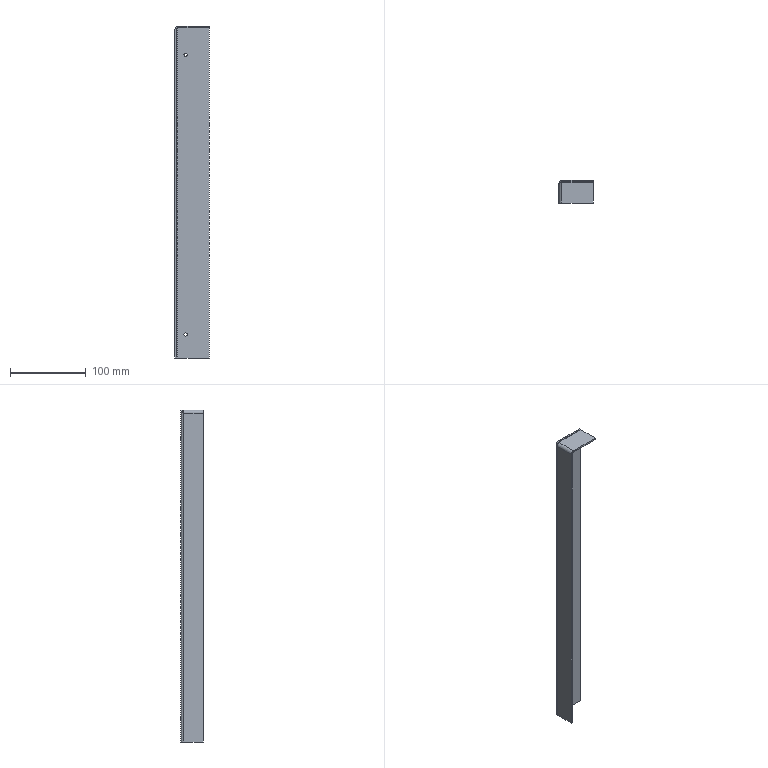Part | STEP file | SYL_0392D6J1SYL0380DJ100-288319 | 1 solid | 26 faces | box 45 x 30 x 438 mm | volume 65045 mm3 | plane 16 | cylinder 8 | spline 2 | commonest cylinder face diameters 4.2 x4 4 x2 8 x2
STEP:
#1=CARTESIAN_POINT('',(-8.5,28.,-190.1));
#2=VERTEX_POINT('',#1);
#3=CARTESIAN_POINT('',(-8.5,30.,-190.1));
#4=VERTEX_POINT('',#3);
#5=CARTESIAN_POINT('',(-8.5,30.,-190.1));
#6=DIRECTION('',(0.,1.,0.));
#7=VECTOR('',#6,1000.);
#8=LINE('',#5,#7);
#9=EDGE_CURVE('',#2,#4,#8,.T.);
#10=ORIENTED_EDGE('',*,*,#9,.F.);
#11=CARTESIAN_POINT('',(-8.5,28.,-185.9));
#12=VERTEX_POINT('',#11);
#13=CARTESIAN_POINT('',(-8.5,28.,-188.));
#14=DIRECTION('',(0.,-1.,0.));
#15=DIRECTION('',(0.,0.,-1.));
#16=AXIS2_PLACEMENT_3D('',#13,#14,#15);
#17=CIRCLE('',#16,2.1);
#18=EDGE_CURVE('',#2,#12,#17,.T.);
#19=ORIENTED_EDGE('',*,*,#18,.T.);
#20=CARTESIAN_POINT('',(-8.5,30.,-185.9));
#21=VERTEX_POINT('',#20);
#22=CARTESIAN_POINT('',(-8.5,30.,-185.9));
#23=DIRECTION('',(0.,1.,0.));
#24=VECTOR('',#23,1000.);
#25=LINE('',#22,#24);
#26=EDGE_CURVE('',#12,#21,#25,.T.);
#27=ORIENTED_EDGE('',*,*,#26,.T.);
#28=CARTESIAN_POINT('',(-8.5,30.,-188.));
#29=DIRECTION('',(0.,-1.,0.));
#30=DIRECTION('',(0.,0.,-1.));
#31=AXIS2_PLACEMENT_3D('',#28,#29,#30);
#32=CIRCLE('',#31,2.1);
#33=EDGE_CURVE('',#4,#21,#32,.T.);
#34=ORIENTED_EDGE('',*,*,#33,.F.);
#35=EDGE_LOOP('',(#10,#19,#27,#34));
#36=FACE_OUTER_BOUND('',#35,.T.);
#37=CARTESIAN_POINT('',(-8.5,30.,-188.));
#38=DIRECTION('',(0.,1.,0.));
#39=DIRECTION('',(0.,0.,1.));
#40=AXIS2_PLACEMENT_3D('',#37,#38,#39);
#41=CYLINDRICAL_SURFACE('',#40,2.1);
#42=ADVANCED_FACE('',(#36),#41,.F.);
#43=CARTESIAN_POINT('',(-8.5,28.,178.9));
#44=VERTEX_POINT('',#43);
#45=CARTESIAN_POINT('',(-8.5,30.,178.9));
#46=VERTEX_POINT('',#45);
#47=CARTESIAN_POINT('',(-8.5,30.,178.9));
#48=DIRECTION('',(0.,1.,0.));
#49=VECTOR('',#48,1000.);
#50=LINE('',#47,#49);
#51=EDGE_CURVE('',#44,#46,#50,.T.);
#52=ORIENTED_EDGE('',*,*,#51,.F.);
#53=CARTESIAN_POINT('',(-8.5,28.,183.1));
#54=VERTEX_POINT('',#53);
#55=CARTESIAN_POINT('',(-8.5,28.,181.));
#56=DIRECTION('',(0.,-1.,0.));
#57=DIRECTION('',(0.,0.,-1.));
#58=AXIS2_PLACEMENT_3D('',#55,#56,#57);
#59=CIRCLE('',#58,2.1);
#60=EDGE_CURVE('',#44,#54,#59,.T.);
#61=ORIENTED_EDGE('',*,*,#60,.T.);
#62=CARTESIAN_POINT('',(-8.5,30.,183.1));
#63=VERTEX_POINT('',#62);
#64=CARTESIAN_POINT('',(-8.5,30.,183.1));
#65=DIRECTION('',(0.,1.,0.));
#66=VECTOR('',#65,1000.);
#67=LINE('',#64,#66);
#68=EDGE_CURVE('',#54,#63,#67,.T.);
#69=ORIENTED_EDGE('',*,*,#68,.T.);
#70=CARTESIAN_POINT('',(-8.5,30.,181.));
#71=DIRECTION('',(0.,-1.,0.));
#72=DIRECTION('',(0.,0.,-1.));
#73=AXIS2_PLACEMENT_3D('',#70,#71,#72);
#74=CIRCLE('',#73,2.1);
#75=EDGE_CURVE('',#46,#63,#74,.T.);
#76=ORIENTED_EDGE('',*,*,#75,.F.);
#77=EDGE_LOOP('',(#52,#61,#69,#76));
#78=FACE_OUTER_BOUND('',#77,.T.);
#79=CARTESIAN_POINT('',(-8.5,30.,181.));
#80=DIRECTION('',(0.,1.,0.));
#81=DIRECTION('',(0.,0.,1.));
#82=AXIS2_PLACEMENT_3D('',#79,#80,#81);
#83=CYLINDRICAL_SURFACE('',#82,2.1);
#84=ADVANCED_FACE('',(#78),#83,.F.);
#85=CARTESIAN_POINT('',(-18.5,28.,219.));
#86=VERTEX_POINT('',#85);
#87=CARTESIAN_POINT('',(-18.5,30.,219.));
#88=VERTEX_POINT('',#87);
#89=CARTESIAN_POINT('',(-18.5,28.,219.));
#90=CARTESIAN_POINT('',(-18.5,30.,219.));
#91=B_SPLINE_CURVE_WITH_KNOTS('',1,(#89,#90),.UNSPECIFIED.,.F.,.F.,(2,2),(0.,1.),.UNSPECIFIED.);
#92=EDGE_CURVE('',#86,#88,#91,.T.);
#93=ORIENTED_EDGE('',*,*,#92,.F.);
#94=CARTESIAN_POINT('',(22.5,28.,219.));
#95=VERTEX_POINT('',#94);
#96=CARTESIAN_POINT('',(22.5,28.,219.));
#97=DIRECTION('',(-1.,0.,0.));
#98=VECTOR('',#97,1000.);
#99=LINE('',#96,#98);
#100=EDGE_CURVE('',#95,#86,#99,.T.);
#101=ORIENTED_EDGE('',*,*,#100,.F.);
#102=CARTESIAN_POINT('',(22.5,30.,219.));
#103=VERTEX_POINT('',#102);
#104=CARTESIAN_POINT('',(22.5,30.,219.));
#105=DIRECTION('',(0.,1.,0.));
#106=VECTOR('',#105,1000.);
#107=LINE('',#104,#106);
#108=EDGE_CURVE('',#95,#103,#107,.T.);
#109=ORIENTED_EDGE('',*,*,#108,.T.);
#110=CARTESIAN_POINT('',(22.5,30.,219.));
#111=DIRECTION('',(-1.,0.,0.));
#112=VECTOR('',#111,1000.);
#113=LINE('',#110,#112);
#114=EDGE_CURVE('',#103,#88,#113,.T.);
#115=ORIENTED_EDGE('',*,*,#114,.T.);
#116=EDGE_LOOP('',(#93,#101,#109,#115));
#117=FACE_OUTER_BOUND('',#116,.T.);
#118=CARTESIAN_POINT('',(22.5,30.,219.));
#119=DIRECTION('',(0.,0.,-1.));
#120=DIRECTION('',(-1.,0.,0.));
#121=AXIS2_PLACEMENT_3D('',#118,#119,#120);
#122=PLANE('',#121);
#123=ADVANCED_FACE('',(#117),#122,.F.);
#124=ORIENTED_EDGE('',*,*,#108,.F.);
#125=CARTESIAN_POINT('',(22.5,28.,-219.));
#126=VERTEX_POINT('',#125);
#127=CARTESIAN_POINT('',(22.5,28.,-219.));
#128=DIRECTION('',(0.,0.,1.));
#129=VECTOR('',#128,1000.);
#130=LINE('',#127,#129);
#131=EDGE_CURVE('',#126,#95,#130,.T.);
#132=ORIENTED_EDGE('',*,*,#131,.F.);
#133=CARTESIAN_POINT('',(22.5,30.,-219.));
#134=VERTEX_POINT('',#133);
#135=CARTESIAN_POINT('',(22.5,30.,-219.));
#136=DIRECTION('',(0.,1.,0.));
#137=VECTOR('',#136,1000.);
#138=LINE('',#135,#137);
#139=EDGE_CURVE('',#126,#134,#138,.T.);
#140=ORIENTED_EDGE('',*,*,#139,.T.);
#141=CARTESIAN_POINT('',(22.5,30.,-219.));
#142=DIRECTION('',(0.,0.,1.));
#143=VECTOR('',#142,1000.);
#144=LINE('',#141,#143);
#145=EDGE_CURVE('',#134,#103,#144,.T.);
#146=ORIENTED_EDGE('',*,*,#145,.T.);
#147=EDGE_LOOP('',(#124,#132,#140,#146));
#148=FACE_OUTER_BOUND('',#147,.T.);
#149=CARTESIAN_POINT('',(22.5,30.,-219.));
#150=DIRECTION('',(-1.,0.,0.));
#151=DIRECTION('',(0.,0.,1.));
#152=AXIS2_PLACEMENT_3D('',#149,#150,#151);
#153=PLANE('',#152);
#154=ADVANCED_FACE('',(#148),#153,.F.);
#155=ORIENTED_EDGE('',*,*,#139,.F.);
#156=CARTESIAN_POINT('',(-18.5,28.,-219.));
#157=VERTEX_POINT('',#156);
#158=CARTESIAN_POINT('',(22.5,28.,-219.));
#159=DIRECTION('',(1.,0.,0.));
#160=VECTOR('',#159,1000.);
#161=LINE('',#158,#160);
#162=EDGE_CURVE('',#157,#126,#161,.T.);
#163=ORIENTED_EDGE('',*,*,#162,.F.);
#164=CARTESIAN_POINT('',(-18.5,30.,-219.));
#165=VERTEX_POINT('',#164);
#166=CARTESIAN_POINT('',(-18.5,30.,-219.));
#167=DIRECTION('',(0.,1.,0.));
#168=VECTOR('',#167,1000.);
#169=LINE('',#166,#168);
#170=EDGE_CURVE('',#157,#165,#169,.T.);
#171=ORIENTED_EDGE('',*,*,#170,.T.);
#172=CARTESIAN_POINT('',(-18.5,30.,-219.));
#173=DIRECTION('',(1.,0.,0.));
#174=VECTOR('',#173,1000.);
#175=LINE('',#172,#174);
#176=EDGE_CURVE('',#165,#134,#175,.T.);
#177=ORIENTED_EDGE('',*,*,#176,.T.);
#178=EDGE_LOOP('',(#155,#163,#171,#177));
#179=FACE_OUTER_BOUND('',#178,.T.);
#180=CARTESIAN_POINT('',(-18.5,30.,-219.));
#181=DIRECTION('',(0.,0.,1.));
#182=DIRECTION('',(1.,0.,0.));
#183=AXIS2_PLACEMENT_3D('',#180,#181,#182);
#184=PLANE('',#183);
#185=ADVANCED_FACE('',(#179),#184,.F.);
#186=ORIENTED_EDGE('',*,*,#170,.F.);
#187=CARTESIAN_POINT('',(-20.5,26.,-219.));
#188=VERTEX_POINT('',#187);
#189=CARTESIAN_POINT('',(-18.5,26.,-219.));
#190=DIRECTION('',(0.,0.,-1.));
#191=DIRECTION('',(-1.,0.,0.));
#192=AXIS2_PLACEMENT_3D('',#189,#190,#191);
#193=CIRCLE('',#192,2.);
#194=EDGE_CURVE('',#188,#157,#193,.T.);
#195=ORIENTED_EDGE('',*,*,#194,.F.);
#196=CARTESIAN_POINT('',(-22.5,26.,-219.));
#197=VERTEX_POINT('',#196);
#198=CARTESIAN_POINT('',(-22.5,26.,-219.));
#199=DIRECTION('',(-1.,0.,0.));
#200=VECTOR('',#199,1000.);
#201=LINE('',#198,#200);
#202=EDGE_CURVE('',#188,#197,#201,.T.);
#203=ORIENTED_EDGE('',*,*,#202,.T.);
#204=CARTESIAN_POINT('',(-18.5,26.,-219.));
#205=DIRECTION('',(0.,0.,-1.));
#206=DIRECTION('',(-1.,0.,0.));
#207=AXIS2_PLACEMENT_3D('',#204,#205,#206);
#208=CIRCLE('',#207,4.);
#209=EDGE_CURVE('',#197,#165,#208,.T.);
#210=ORIENTED_EDGE('',*,*,#209,.T.);
#211=EDGE_LOOP('',(#186,#195,#203,#210));
#212=FACE_OUTER_BOUND('',#211,.T.);
#213=CARTESIAN_POINT('',(-18.5,26.,-219.));
#214=DIRECTION('',(0.,0.,1.));
#215=DIRECTION('',(1.,0.,0.));
#216=AXIS2_PLACEMENT_3D('',#213,#214,#215);
#217=PLANE('',#216);
#218=ADVANCED_FACE('',(#212),#217,.F.);
#219=ORIENTED_EDGE('',*,*,#202,.F.);
#220=CARTESIAN_POINT('',(-20.5,0.,-219.));
#221=VERTEX_POINT('',#220);
#222=CARTESIAN_POINT('',(-20.5,30.,-219.));
#223=DIRECTION('',(0.,1.,0.));
#224=VECTOR('',#223,1000.);
#225=LINE('',#222,#224);
#226=EDGE_CURVE('',#221,#188,#225,.T.);
#227=ORIENTED_EDGE('',*,*,#226,.F.);
#228=CARTESIAN_POINT('',(-22.5,0.,-219.));
#229=VERTEX_POINT('',#228);
#230=CARTESIAN_POINT('',(-22.5,0.,-219.));
#231=DIRECTION('',(-1.,0.,0.));
#232=VECTOR('',#231,1000.);
#233=LINE('',#230,#232);
#234=EDGE_CURVE('',#221,#229,#233,.T.);
#235=ORIENTED_EDGE('',*,*,#234,.T.);
#236=CARTESIAN_POINT('',(-22.5,0.,-219.));
#237=DIRECTION('',(0.,1.,0.));
#238=VECTOR('',#237,1000.);
#239=LINE('',#236,#238);
#240=EDGE_CURVE('',#229,#197,#239,.T.);
#241=ORIENTED_EDGE('',*,*,#240,.T.);
#242=EDGE_LOOP('',(#219,#227,#235,#241));
#243=FACE_OUTER_BOUND('',#242,.T.);
#244=CARTESIAN_POINT('',(-22.5,0.,-219.));
#245=DIRECTION('',(0.,0.,1.));
#246=DIRECTION('',(0.,1.,0.));
#247=AXIS2_PLACEMENT_3D('',#244,#245,#246);
#248=PLANE('',#247);
#249=ADVANCED_FACE('',(#243),#248,.F.);
#250=ORIENTED_EDGE('',*,*,#234,.F.);
#251=CARTESIAN_POINT('',(-20.5,0.,215.));
#252=VERTEX_POINT('',#251);
#253=CARTESIAN_POINT('',(-20.5,0.,-219.));
#254=DIRECTION('',(0.,0.,-1.));
#255=VECTOR('',#254,1000.);
#256=LINE('',#253,#255);
#257=EDGE_CURVE('',#252,#221,#256,.T.);
#258=ORIENTED_EDGE('',*,*,#257,.F.);
#259=CARTESIAN_POINT('',(-22.5,0.,215.));
#260=VERTEX_POINT('',#259);
#261=CARTESIAN_POINT('',(-22.5,0.,215.));
#262=DIRECTION('',(-1.,0.,0.));
#263=VECTOR('',#262,1000.);
#264=LINE('',#261,#263);
#265=EDGE_CURVE('',#252,#260,#264,.T.);
#266=ORIENTED_EDGE('',*,*,#265,.T.);
#267=CARTESIAN_POINT('',(-22.5,0.,215.));
#268=DIRECTION('',(0.,0.,-1.));
#269=VECTOR('',#268,1000.);
#270=LINE('',#267,#269);
#271=EDGE_CURVE('',#260,#229,#270,.T.);
#272=ORIENTED_EDGE('',*,*,#271,.T.);
#273=EDGE_LOOP('',(#250,#258,#266,#272));
#274=FACE_OUTER_BOUND('',#273,.T.);
#275=CARTESIAN_POINT('',(-22.5,0.,215.));
#276=DIRECTION('',(0.,1.,0.));
#277=DIRECTION('',(0.,0.,-1.));
#278=AXIS2_PLACEMENT_3D('',#275,#276,#277);
#279=PLANE('',#278);
#280=ADVANCED_FACE('',(#274),#279,.F.);
#281=ORIENTED_EDGE('',*,*,#265,.F.);
#282=CARTESIAN_POINT('',(-18.5,0.,217.));
#283=VERTEX_POINT('',#282);
#284=CARTESIAN_POINT('',(-18.5,0.,215.));
#285=DIRECTION('',(0.,-1.,0.));
#286=DIRECTION('',(0.,0.,-1.));
#287=AXIS2_PLACEMENT_3D('',#284,#285,#286);
#288=CIRCLE('',#287,2.);
#289=EDGE_CURVE('',#283,#252,#288,.T.);
#290=ORIENTED_EDGE('',*,*,#289,.F.);
#291=CARTESIAN_POINT('',(-18.5,0.,219.));
#292=VERTEX_POINT('',#291);
#293=CARTESIAN_POINT('',(-18.5,0.,219.));
#294=DIRECTION('',(0.,0.,1.));
#295=VECTOR('',#294,1000.);
#296=LINE('',#293,#295);
#297=EDGE_CURVE('',#283,#292,#296,.T.);
#298=ORIENTED_EDGE('',*,*,#297,.T.);
#299=CARTESIAN_POINT('',(-18.5,0.,215.));
#300=DIRECTION('',(0.,-1.,0.));
#301=DIRECTION('',(0.,0.,1.));
#302=AXIS2_PLACEMENT_3D('',#299,#300,#301);
#303=CIRCLE('',#302,4.);
#304=EDGE_CURVE('',#292,#260,#303,.T.);
#305=ORIENTED_EDGE('',*,*,#304,.T.);
#306=EDGE_LOOP('',(#281,#290,#298,#305));
#307=FACE_OUTER_BOUND('',#306,.T.);
#308=CARTESIAN_POINT('',(-18.5,0.,215.));
#309=DIRECTION('',(0.,1.,0.));
#310=DIRECTION('',(0.,0.,1.));
#311=AXIS2_PLACEMENT_3D('',#308,#309,#310);
#312=PLANE('',#311);
#313=ADVANCED_FACE('',(#307),#312,.F.);
#314=ORIENTED_EDGE('',*,*,#297,.F.);
#315=CARTESIAN_POINT('',(22.5,0.,217.));
#316=VERTEX_POINT('',#315);
#317=CARTESIAN_POINT('',(-22.5,0.,217.));
#318=DIRECTION('',(-1.,0.,0.));
#319=VECTOR('',#318,1000.);
#320=LINE('',#317,#319);
#321=EDGE_CURVE('',#316,#283,#320,.T.);
#322=ORIENTED_EDGE('',*,*,#321,.F.);
#323=CARTESIAN_POINT('',(22.5,0.,219.));
#324=VERTEX_POINT('',#323);
#325=CARTESIAN_POINT('',(22.5,0.,219.));
#326=DIRECTION('',(0.,0.,1.));
#327=VECTOR('',#326,1000.);
#328=LINE('',#325,#327);
#329=EDGE_CURVE('',#316,#324,#328,.T.);
#330=ORIENTED_EDGE('',*,*,#329,.T.);
#331=CARTESIAN_POINT('',(22.5,0.,219.));
#332=DIRECTION('',(-1.,0.,0.));
#333=VECTOR('',#332,1000.);
#334=LINE('',#331,#333);
#335=EDGE_CURVE('',#324,#292,#334,.T.);
#336=ORIENTED_EDGE('',*,*,#335,.T.);
#337=EDGE_LOOP('',(#314,#322,#330,#336));
#338=FACE_OUTER_BOUND('',#337,.T.);
#339=CARTESIAN_POINT('',(22.5,0.,219.));
#340=DIRECTION('',(0.,1.,0.));
#341=DIRECTION('',(-1.,0.,0.));
#342=AXIS2_PLACEMENT_3D('',#339,#340,#341);
#343=PLANE('',#342);
#344=ADVANCED_FACE('',(#338),#343,.F.);
#345=ORIENTED_EDGE('',*,*,#329,.F.);
#346=CARTESIAN_POINT('',(22.5,27.5,217.));
#347=VERTEX_POINT('',#346);
#348=CARTESIAN_POINT('',(22.5,0.,217.));
#349=DIRECTION('',(0.,-1.,0.));
#350=VECTOR('',#349,1000.);
#351=LINE('',#348,#350);
#352=EDGE_CURVE('',#347,#316,#351,.T.);
#353=ORIENTED_EDGE('',*,*,#352,.F.);
#354=CARTESIAN_POINT('',(22.5,27.5,219.));
#355=VERTEX_POINT('',#354);
#356=CARTESIAN_POINT('',(22.5,27.5,219.));
#357=DIRECTION('',(0.,0.,1.));
#358=VECTOR('',#357,1000.);
#359=LINE('',#356,#358);
#360=EDGE_CURVE('',#347,#355,#359,.T.);
#361=ORIENTED_EDGE('',*,*,#360,.T.);
#362=CARTESIAN_POINT('',(22.5,27.5,219.));
#363=DIRECTION('',(0.,-1.,0.));
#364=VECTOR('',#363,1000.);
#365=LINE('',#362,#364);
#366=EDGE_CURVE('',#355,#324,#365,.T.);
#367=ORIENTED_EDGE('',*,*,#366,.T.);
#368=EDGE_LOOP('',(#345,#353,#361,#367));
#369=FACE_OUTER_BOUND('',#368,.T.);
#370=CARTESIAN_POINT('',(22.5,27.5,219.));
#371=DIRECTION('',(-1.,0.,0.));
#372=DIRECTION('',(0.,-1.,0.));
#373=AXIS2_PLACEMENT_3D('',#370,#371,#372);
#374=PLANE('',#373);
#375=ADVANCED_FACE('',(#369),#374,.F.);
#376=ORIENTED_EDGE('',*,*,#360,.F.);
#377=CARTESIAN_POINT('',(-18.5,27.5,217.));
#378=VERTEX_POINT('',#377);
#379=CARTESIAN_POINT('',(-22.5,27.5,217.));
#380=DIRECTION('',(1.,0.,0.));
#381=VECTOR('',#380,1000.);
#382=LINE('',#379,#381);
#383=EDGE_CURVE('',#378,#347,#382,.T.);
#384=ORIENTED_EDGE('',*,*,#383,.F.);
#385=CARTESIAN_POINT('',(-18.5,27.5,219.));
#386=VERTEX_POINT('',#385);
#387=CARTESIAN_POINT('',(-18.5,27.5,217.));
#388=CARTESIAN_POINT('',(-18.5,27.5,217.667));
#389=CARTESIAN_POINT('',(-18.5,27.5,218.333));
#390=CARTESIAN_POINT('',(-18.5,27.5,219.));
#391=B_SPLINE_CURVE_WITH_KNOTS('',3,(#387,#388,#389,#390),.UNSPECIFIED.,.F.,.F.,(4,4),(0.,1.),.UNSPECIFIED.);
#392=EDGE_CURVE('',#378,#386,#391,.T.);
#393=ORIENTED_EDGE('',*,*,#392,.T.);
#394=CARTESIAN_POINT('',(-18.5,27.5,219.));
#395=DIRECTION('',(1.,0.,0.));
#396=VECTOR('',#395,1000.);
#397=LINE('',#394,#396);
#398=EDGE_CURVE('',#386,#355,#397,.T.);
#399=ORIENTED_EDGE('',*,*,#398,.T.);
#400=EDGE_LOOP('',(#376,#384,#393,#399));
#401=FACE_OUTER_BOUND('',#400,.T.);
#402=CARTESIAN_POINT('',(-18.5,27.5,219.));
#403=DIRECTION('',(0.,-1.,0.));
#404=DIRECTION('',(1.,0.,0.));
#405=AXIS2_PLACEMENT_3D('',#402,#403,#404);
#406=PLANE('',#405);
#407=ADVANCED_FACE('',(#401),#406,.F.);
#408=ORIENTED_EDGE('',*,*,#392,.F.);
#409=CARTESIAN_POINT('',(-20.5,26.,215.));
#410=VERTEX_POINT('',#409);
#411=CARTESIAN_POINT('',(-18.5,27.5,217.));
#412=CARTESIAN_POINT('',(-18.762,27.375,217.));
#413=CARTESIAN_POINT('',(-19.023,27.25,216.948));
#414=CARTESIAN_POINT('',(-19.507,27.,216.748));
#415=CARTESIAN_POINT('',(-19.729,26.875,216.599));
#416=CARTESIAN_POINT('',(-20.099,26.625,216.229));
#417=CARTESIAN_POINT('',(-20.248,26.5,216.007));
#418=CARTESIAN_POINT('',(-20.448,26.25,215.523));
#419=CARTESIAN_POINT('',(-20.5,26.125,215.262));
#420=CARTESIAN_POINT('',(-20.5,26.,215.));
#421=B_SPLINE_CURVE_WITH_KNOTS('',3,(#411,#412,#413,#414,#415,#416,#417,#418,#419,#420),.UNSPECIFIED.,.F.,.F.,(4,2,2,2,4),(0.,0.25,0.5,0.75,1.),.UNSPECIFIED.);
#422=EDGE_CURVE('',#378,#410,#421,.T.);
#423=ORIENTED_EDGE('',*,*,#422,.T.);
#424=CARTESIAN_POINT('',(-22.5,26.,215.));
#425=VERTEX_POINT('',#424);
#426=CARTESIAN_POINT('',(-20.5,26.,215.));
#427=CARTESIAN_POINT('',(-22.5,26.,215.));
#428=B_SPLINE_CURVE_WITH_KNOTS('',1,(#426,#427),.UNSPECIFIED.,.F.,.F.,(2,2),(0.,1.),.UNSPECIFIED.);
#429=EDGE_CURVE('',#410,#425,#428,.T.);
#430=ORIENTED_EDGE('',*,*,#429,.T.);
#431=CARTESIAN_POINT('',(-18.5,27.5,219.));
#432=CARTESIAN_POINT('',(-19.024,27.375,219.));
#433=CARTESIAN_POINT('',(-19.547,27.25,218.896));
#434=CARTESIAN_POINT('',(-20.514,27.,218.495));
#435=CARTESIAN_POINT('',(-20.958,26.875,218.199));
#436=CARTESIAN_POINT('',(-21.699,26.625,217.458));
#437=CARTESIAN_POINT('',(-21.995,26.5,217.014));
#438=CARTESIAN_POINT('',(-22.396,26.25,216.047));
#439=CARTESIAN_POINT('',(-22.5,26.125,215.524));
#440=CARTESIAN_POINT('',(-22.5,26.,215.));
#441=B_SPLINE_CURVE_WITH_KNOTS('',3,(#431,#432,#433,#434,#435,#436,#437,#438,#439,#440),.UNSPECIFIED.,.F.,.F.,(4,2,2,2,4),(0.,0.25,0.5,0.75,1.),.UNSPECIFIED.);
#442=EDGE_CURVE('',#386,#425,#441,.T.);
#443=ORIENTED_EDGE('',*,*,#442,.F.);
#444=EDGE_LOOP('',(#408,#423,#430,#443));
#445=FACE_OUTER_BOUND('',#444,.T.);
#446=CARTESIAN_POINT('',(-18.5,27.5,219.));
#447=CARTESIAN_POINT('',(-19.024,27.375,219.));
#448=CARTESIAN_POINT('',(-19.547,27.25,218.896));
#449=CARTESIAN_POINT('',(-20.514,27.,218.495));
#450=CARTESIAN_POINT('',(-20.958,26.875,218.199));
#451=CARTESIAN_POINT('',(-21.699,26.625,217.458));
#452=CARTESIAN_POINT('',(-21.995,26.5,217.014));
#453=CARTESIAN_POINT('',(-22.396,26.25,216.047));
#454=CARTESIAN_POINT('',(-22.5,26.125,215.524));
#455=CARTESIAN_POINT('',(-22.5,26.,215.));
#456=CARTESIAN_POINT('',(-18.5,27.5,217.));
#457=CARTESIAN_POINT('',(-18.762,27.375,217.));
#458=CARTESIAN_POINT('',(-19.023,27.25,216.948));
#459=CARTESIAN_POINT('',(-19.507,27.,216.748));
#460=CARTESIAN_POINT('',(-19.729,26.875,216.599));
#461=CARTESIAN_POINT('',(-20.099,26.625,216.229));
#462=CARTESIAN_POINT('',(-20.248,26.5,216.007));
#463=CARTESIAN_POINT('',(-20.448,26.25,215.523));
#464=CARTESIAN_POINT('',(-20.5,26.125,215.262));
#465=CARTESIAN_POINT('',(-20.5,26.,215.));
#466=B_SPLINE_SURFACE_WITH_KNOTS('',1,3,((#446,#447,#448,#449,#450,#451,#452,#453,#454,#455),(#456,#457,#458,#459,#460,#461,#462,#463,#464,#465)),.UNSPECIFIED.,.F.,.F.,.F.,(2,2),(4,2,2,2,4),(0.,1.),(0.,0.25,0.5,0.75,1.),.UNSPECIFIED.);
#467=ADVANCED_FACE('',(#445),#466,.T.);
#468=CARTESIAN_POINT('',(-8.5,28.,181.));
#469=DIRECTION('',(0.,-1.,0.));
#470=DIRECTION('',(0.,0.,-1.));
#471=AXIS2_PLACEMENT_3D('',#468,#469,#470);
#472=CIRCLE('',#471,2.1);
#473=EDGE_CURVE('',#54,#44,#472,.T.);
#474=ORIENTED_EDGE('',*,*,#473,.T.);
#475=ORIENTED_EDGE('',*,*,#51,.T.);
#476=CARTESIAN_POINT('',(-8.5,30.,181.));
#477=DIRECTION('',(0.,-1.,0.));
#478=DIRECTION('',(0.,0.,1.));
#479=AXIS2_PLACEMENT_3D('',#476,#477,#478);
#480=CIRCLE('',#479,2.1);
#481=EDGE_CURVE('',#63,#46,#480,.T.);
#482=ORIENTED_EDGE('',*,*,#481,.F.);
#483=ORIENTED_EDGE('',*,*,#68,.F.);
#484=EDGE_LOOP('',(#474,#475,#482,#483));
#485=FACE_OUTER_BOUND('',#484,.T.);
#486=CARTESIAN_POINT('',(-8.5,30.,181.));
#487=DIRECTION('',(0.,1.,0.));
#488=DIRECTION('',(0.,0.,1.));
#489=AXIS2_PLACEMENT_3D('',#486,#487,#488);
#490=CYLINDRICAL_SURFACE('',#489,2.1);
#491=ADVANCED_FACE('',(#485),#490,.F.);
#492=CARTESIAN_POINT('',(-8.5,28.,-188.));
#493=DIRECTION('',(0.,-1.,0.));
#494=DIRECTION('',(0.,0.,-1.));
#495=AXIS2_PLACEMENT_3D('',#492,#493,#494);
#496=CIRCLE('',#495,2.1);
#497=EDGE_CURVE('',#12,#2,#496,.T.);
#498=ORIENTED_EDGE('',*,*,#497,.T.);
#499=ORIENTED_EDGE('',*,*,#9,.T.);
#500=CARTESIAN_POINT('',(-8.5,30.,-188.));
#501=DIRECTION('',(0.,-1.,0.));
#502=DIRECTION('',(0.,0.,1.));
#503=AXIS2_PLACEMENT_3D('',#500,#501,#502);
#504=CIRCLE('',#503,2.1);
#505=EDGE_CURVE('',#21,#4,#504,.T.);
#506=ORIENTED_EDGE('',*,*,#505,.F.);
#507=ORIENTED_EDGE('',*,*,#26,.F.);
#508=EDGE_LOOP('',(#498,#499,#506,#507));
#509=FACE_OUTER_BOUND('',#508,.T.);
#510=CARTESIAN_POINT('',(-8.5,30.,-188.));
#511=DIRECTION('',(0.,1.,0.));
#512=DIRECTION('',(0.,0.,1.));
#513=AXIS2_PLACEMENT_3D('',#510,#511,#512);
#514=CYLINDRICAL_SURFACE('',#513,2.1);
#515=ADVANCED_FACE('',(#509),#514,.F.);
#516=CARTESIAN_POINT('',(-20.5,26.,215.));
#517=CARTESIAN_POINT('',(-20.5,26.262,215.333));
#518=CARTESIAN_POINT('',(-20.448,26.523,215.667));
#519=CARTESIAN_POINT('',(-20.248,27.007,216.333));
#520=CARTESIAN_POINT('',(-20.099,27.229,216.667));
#521=CARTESIAN_POINT('',(-19.729,27.599,217.333));
#522=CARTESIAN_POINT('',(-19.507,27.748,217.667));
#523=CARTESIAN_POINT('',(-19.023,27.948,218.333));
#524=CARTESIAN_POINT('',(-18.762,28.,218.667));
#525=CARTESIAN_POINT('',(-18.5,28.,219.));
#526=B_SPLINE_CURVE_WITH_KNOTS('',3,(#516,#517,#518,#519,#520,#521,#522,#523,#524,#525),.UNSPECIFIED.,.F.,.F.,(4,2,2,2,4),(0.,0.25,0.5,0.75,1.),.UNSPECIFIED.);
#527=EDGE_CURVE('',#410,#86,#526,.T.);
#528=ORIENTED_EDGE('',*,*,#527,.T.);
#529=ORIENTED_EDGE('',*,*,#92,.T.);
#530=CARTESIAN_POINT('',(-22.5,26.,215.));
#531=CARTESIAN_POINT('',(-22.5,26.524,215.333));
#532=CARTESIAN_POINT('',(-22.396,27.047,215.667));
#533=CARTESIAN_POINT('',(-21.995,28.014,216.333));
#534=CARTESIAN_POINT('',(-21.699,28.458,216.667));
#535=CARTESIAN_POINT('',(-20.958,29.199,217.333));
#536=CARTESIAN_POINT('',(-20.514,29.495,217.667));
#537=CARTESIAN_POINT('',(-19.547,29.896,218.333));
#538=CARTESIAN_POINT('',(-19.024,30.,218.667));
#539=CARTESIAN_POINT('',(-18.5,30.,219.));
#540=B_SPLINE_CURVE_WITH_KNOTS('',3,(#530,#531,#532,#533,#534,#535,#536,#537,#538,#539),.UNSPECIFIED.,.F.,.F.,(4,2,2,2,4),(0.,0.25,0.5,0.75,1.),.UNSPECIFIED.);
#541=EDGE_CURVE('',#425,#88,#540,.T.);
#542=ORIENTED_EDGE('',*,*,#541,.F.);
#543=ORIENTED_EDGE('',*,*,#429,.F.);
#544=EDGE_LOOP('',(#528,#529,#542,#543));
#545=FACE_OUTER_BOUND('',#544,.T.);
#546=CARTESIAN_POINT('',(-22.5,26.,215.));
#547=CARTESIAN_POINT('',(-22.5,26.524,215.333));
#548=CARTESIAN_POINT('',(-22.396,27.047,215.667));
#549=CARTESIAN_POINT('',(-21.995,28.014,216.333));
#550=CARTESIAN_POINT('',(-21.699,28.458,216.667));
#551=CARTESIAN_POINT('',(-20.958,29.199,217.333));
#552=CARTESIAN_POINT('',(-20.514,29.495,217.667));
#553=CARTESIAN_POINT('',(-19.547,29.896,218.333));
#554=CARTESIAN_POINT('',(-19.024,30.,218.667));
#555=CARTESIAN_POINT('',(-18.5,30.,219.));
#556=CARTESIAN_POINT('',(-20.5,26.,215.));
#557=CARTESIAN_POINT('',(-20.5,26.262,215.333));
#558=CARTESIAN_POINT('',(-20.448,26.523,215.667));
#559=CARTESIAN_POINT('',(-20.248,27.007,216.333));
#560=CARTESIAN_POINT('',(-20.099,27.229,216.667));
#561=CARTESIAN_POINT('',(-19.729,27.599,217.333));
#562=CARTESIAN_POINT('',(-19.507,27.748,217.667));
#563=CARTESIAN_POINT('',(-19.023,27.948,218.333));
#564=CARTESIAN_POINT('',(-18.762,28.,218.667));
#565=CARTESIAN_POINT('',(-18.5,28.,219.));
#566=B_SPLINE_SURFACE_WITH_KNOTS('',1,3,((#546,#547,#548,#549,#550,#551,#552,#553,#554,#555),(#556,#557,#558,#559,#560,#561,#562,#563,#564,#565)),.UNSPECIFIED.,.F.,.F.,.F.,(2,2),(4,2,2,2,4),(0.,1.),(0.,0.25,0.5,0.75,1.),.UNSPECIFIED.);
#567=ADVANCED_FACE('',(#545),#566,.T.);
#568=ORIENTED_EDGE('',*,*,#442,.T.);
#569=CARTESIAN_POINT('',(-22.5,26.,215.));
#570=DIRECTION('',(0.,-1.,0.));
#571=VECTOR('',#570,1000.);
#572=LINE('',#569,#571);
#573=EDGE_CURVE('',#425,#260,#572,.T.);
#574=ORIENTED_EDGE('',*,*,#573,.T.);
#575=ORIENTED_EDGE('',*,*,#304,.F.);
#576=CARTESIAN_POINT('',(-18.5,0.,219.));
#577=DIRECTION('',(0.,1.,0.));
#578=VECTOR('',#577,1000.);
#579=LINE('',#576,#578);
#580=EDGE_CURVE('',#292,#386,#579,.T.);
#581=ORIENTED_EDGE('',*,*,#580,.T.);
#582=EDGE_LOOP('',(#568,#574,#575,#581));
#583=FACE_OUTER_BOUND('',#582,.T.);
#584=CARTESIAN_POINT('',(-18.5,26.,215.));
#585=DIRECTION('',(0.,-1.,0.));
#586=DIRECTION('',(0.,0.,-1.));
#587=AXIS2_PLACEMENT_3D('',#584,#585,#586);
#588=CYLINDRICAL_SURFACE('',#587,4.);
#589=ADVANCED_FACE('',(#583),#588,.T.);
#590=ORIENTED_EDGE('',*,*,#398,.F.);
#591=ORIENTED_EDGE('',*,*,#580,.F.);
#592=ORIENTED_EDGE('',*,*,#335,.F.);
#593=ORIENTED_EDGE('',*,*,#366,.F.);
#594=EDGE_LOOP('',(#590,#591,#592,#593));
#595=FACE_OUTER_BOUND('',#594,.T.);
#596=CARTESIAN_POINT('',(-22.5,0.,219.));
#597=DIRECTION('',(0.,0.,1.));
#598=DIRECTION('',(1.,0.,0.));
#599=AXIS2_PLACEMENT_3D('',#596,#597,#598);
#600=PLANE('',#599);
#601=ADVANCED_FACE('',(#595),#600,.T.);
#602=ORIENTED_EDGE('',*,*,#541,.T.);
#603=CARTESIAN_POINT('',(-18.5,30.,219.));
#604=DIRECTION('',(0.,0.,-1.));
#605=VECTOR('',#604,1000.);
#606=LINE('',#603,#605);
#607=EDGE_CURVE('',#88,#165,#606,.T.);
#608=ORIENTED_EDGE('',*,*,#607,.T.);
#609=ORIENTED_EDGE('',*,*,#209,.F.);
#610=CARTESIAN_POINT('',(-22.5,26.,-219.));
#611=DIRECTION('',(0.,0.,1.));
#612=VECTOR('',#611,1000.);
#613=LINE('',#610,#612);
#614=EDGE_CURVE('',#197,#425,#613,.T.);
#615=ORIENTED_EDGE('',*,*,#614,.T.);
#616=EDGE_LOOP('',(#602,#608,#609,#615));
#617=FACE_OUTER_BOUND('',#616,.T.);
#618=CARTESIAN_POINT('',(-18.5,26.,-219.));
#619=DIRECTION('',(0.,0.,-1.));
#620=DIRECTION('',(-1.,0.,0.));
#621=AXIS2_PLACEMENT_3D('',#618,#619,#620);
#622=CYLINDRICAL_SURFACE('',#621,4.);
#623=ADVANCED_FACE('',(#617),#622,.T.);
#624=ORIENTED_EDGE('',*,*,#573,.F.);
#625=ORIENTED_EDGE('',*,*,#614,.F.);
#626=ORIENTED_EDGE('',*,*,#240,.F.);
#627=ORIENTED_EDGE('',*,*,#271,.F.);
#628=EDGE_LOOP('',(#624,#625,#626,#627));
#629=FACE_OUTER_BOUND('',#628,.T.);
#630=CARTESIAN_POINT('',(-22.5,30.,-219.));
#631=DIRECTION('',(-1.,0.,0.));
#632=DIRECTION('',(0.,0.,1.));
#633=AXIS2_PLACEMENT_3D('',#630,#631,#632);
#634=PLANE('',#633);
#635=ADVANCED_FACE('',(#629),#634,.T.);
#636=ORIENTED_EDGE('',*,*,#75,.T.);
#637=ORIENTED_EDGE('',*,*,#481,.T.);
#638=EDGE_LOOP('',(#636,#637));
#639=FACE_BOUND('',#638,.T.);
#640=ORIENTED_EDGE('',*,*,#33,.T.);
#641=ORIENTED_EDGE('',*,*,#505,.T.);
#642=EDGE_LOOP('',(#640,#641));
#643=FACE_BOUND('',#642,.T.);
#644=ORIENTED_EDGE('',*,*,#114,.F.);
#645=ORIENTED_EDGE('',*,*,#145,.F.);
#646=ORIENTED_EDGE('',*,*,#176,.F.);
#647=ORIENTED_EDGE('',*,*,#607,.F.);
#648=EDGE_LOOP('',(#644,#645,#646,#647));
#649=FACE_OUTER_BOUND('',#648,.T.);
#650=CARTESIAN_POINT('',(22.5,30.,-219.));
#651=DIRECTION('',(0.,1.,0.));
#652=DIRECTION('',(1.,0.,0.));
#653=AXIS2_PLACEMENT_3D('',#650,#651,#652);
#654=PLANE('',#653);
#655=ADVANCED_FACE('',(#639,#643,#649),#654,.T.);
#656=ORIENTED_EDGE('',*,*,#422,.F.);
#657=CARTESIAN_POINT('',(-18.5,26.,217.));
#658=DIRECTION('',(0.,1.,0.));
#659=VECTOR('',#658,1000.);
#660=LINE('',#657,#659);
#661=EDGE_CURVE('',#283,#378,#660,.T.);
#662=ORIENTED_EDGE('',*,*,#661,.F.);
#663=ORIENTED_EDGE('',*,*,#289,.T.);
#664=CARTESIAN_POINT('',(-20.5,26.,215.));
#665=DIRECTION('',(0.,-1.,0.));
#666=VECTOR('',#665,1000.);
#667=LINE('',#664,#666);
#668=EDGE_CURVE('',#410,#252,#667,.T.);
#669=ORIENTED_EDGE('',*,*,#668,.F.);
#670=EDGE_LOOP('',(#656,#662,#663,#669));
#671=FACE_OUTER_BOUND('',#670,.T.);
#672=CARTESIAN_POINT('',(-18.5,26.,215.));
#673=DIRECTION('',(0.,-1.,0.));
#674=DIRECTION('',(0.,0.,-1.));
#675=AXIS2_PLACEMENT_3D('',#672,#673,#674);
#676=CYLINDRICAL_SURFACE('',#675,2.);
#677=ADVANCED_FACE('',(#671),#676,.F.);
#678=ORIENTED_EDGE('',*,*,#383,.T.);
#679=ORIENTED_EDGE('',*,*,#352,.T.);
#680=ORIENTED_EDGE('',*,*,#321,.T.);
#681=ORIENTED_EDGE('',*,*,#661,.T.);
#682=EDGE_LOOP('',(#678,#679,#680,#681));
#683=FACE_OUTER_BOUND('',#682,.T.);
#684=CARTESIAN_POINT('',(-22.5,0.,217.));
#685=DIRECTION('',(0.,0.,1.));
#686=DIRECTION('',(1.,0.,0.));
#687=AXIS2_PLACEMENT_3D('',#684,#685,#686);
#688=PLANE('',#687);
#689=ADVANCED_FACE('',(#683),#688,.F.);
#690=ORIENTED_EDGE('',*,*,#527,.F.);
#691=CARTESIAN_POINT('',(-20.5,26.,-219.));
#692=DIRECTION('',(0.,0.,1.));
#693=VECTOR('',#692,1000.);
#694=LINE('',#691,#693);
#695=EDGE_CURVE('',#188,#410,#694,.T.);
#696=ORIENTED_EDGE('',*,*,#695,.F.);
#697=ORIENTED_EDGE('',*,*,#194,.T.);
#698=CARTESIAN_POINT('',(-18.5,28.,-219.));
#699=DIRECTION('',(0.,0.,-1.));
#700=VECTOR('',#699,1000.);
#701=LINE('',#698,#700);
#702=EDGE_CURVE('',#86,#157,#701,.T.);
#703=ORIENTED_EDGE('',*,*,#702,.F.);
#704=EDGE_LOOP('',(#690,#696,#697,#703));
#705=FACE_OUTER_BOUND('',#704,.T.);
#706=CARTESIAN_POINT('',(-18.5,26.,-219.));
#707=DIRECTION('',(0.,0.,-1.));
#708=DIRECTION('',(-1.,0.,0.));
#709=AXIS2_PLACEMENT_3D('',#706,#707,#708);
#710=CYLINDRICAL_SURFACE('',#709,2.);
#711=ADVANCED_FACE('',(#705),#710,.F.);
#712=ORIENTED_EDGE('',*,*,#668,.T.);
#713=ORIENTED_EDGE('',*,*,#257,.T.);
#714=ORIENTED_EDGE('',*,*,#226,.T.);
#715=ORIENTED_EDGE('',*,*,#695,.T.);
#716=EDGE_LOOP('',(#712,#713,#714,#715));
#717=FACE_OUTER_BOUND('',#716,.T.);
#718=CARTESIAN_POINT('',(-20.5,30.,-219.));
#719=DIRECTION('',(-1.,0.,0.));
#720=DIRECTION('',(0.,0.,1.));
#721=AXIS2_PLACEMENT_3D('',#718,#719,#720);
#722=PLANE('',#721);
#723=ADVANCED_FACE('',(#717),#722,.F.);
#724=ORIENTED_EDGE('',*,*,#60,.F.);
#725=ORIENTED_EDGE('',*,*,#473,.F.);
#726=EDGE_LOOP('',(#724,#725));
#727=FACE_BOUND('',#726,.T.);
#728=ORIENTED_EDGE('',*,*,#18,.F.);
#729=ORIENTED_EDGE('',*,*,#497,.F.);
#730=EDGE_LOOP('',(#728,#729));
#731=FACE_BOUND('',#730,.T.);
#732=ORIENTED_EDGE('',*,*,#100,.T.);
#733=ORIENTED_EDGE('',*,*,#702,.T.);
#734=ORIENTED_EDGE('',*,*,#162,.T.);
#735=ORIENTED_EDGE('',*,*,#131,.T.);
#736=EDGE_LOOP('',(#732,#733,#734,#735));
#737=FACE_OUTER_BOUND('',#736,.T.);
#738=CARTESIAN_POINT('',(22.5,28.,-219.));
#739=DIRECTION('',(0.,1.,0.));
#740=DIRECTION('',(1.,0.,0.));
#741=AXIS2_PLACEMENT_3D('',#738,#739,#740);
#742=PLANE('',#741);
#743=ADVANCED_FACE('',(#727,#731,#737),#742,.F.);
#744=CLOSED_SHELL('',(#42,#84,#123,#154,#185,#218,#249,#280,#313,#344,#375,#407,#467,#491,#515,#567,#589,#601,#623,#635,#655,#677,#689,#711,#723,#743));
#745=MANIFOLD_SOLID_BREP('',#744);
#746=CARTESIAN_POINT('',(0.,0.,0.));
#747=DIRECTION('',(0.,0.,1.));
#748=DIRECTION('',(1.,0.,0.));
#749=AXIS2_PLACEMENT_3D('',#746,#747,#748);
#750=(LENGTH_UNIT()NAMED_UNIT(*)SI_UNIT(.MILLI.,.METRE.));
#751=UNCERTAINTY_MEASURE_WITH_UNIT(LENGTH_MEASURE(0.00001),#750,'','');
#752=(NAMED_UNIT(*)PLANE_ANGLE_UNIT()SI_UNIT($,.RADIAN.));
#753=(NAMED_UNIT(*)SI_UNIT($,.STERADIAN.)SOLID_ANGLE_UNIT());
#754=(GEOMETRIC_REPRESENTATION_CONTEXT(3)GLOBAL_UNCERTAINTY_ASSIGNED_CONTEXT((#751))GLOBAL_UNIT_ASSIGNED_CONTEXT((#750,#752,#753))REPRESENTATION_CONTEXT('',''));
#755=ADVANCED_BREP_SHAPE_REPRESENTATION('',(#745,#749),#754);